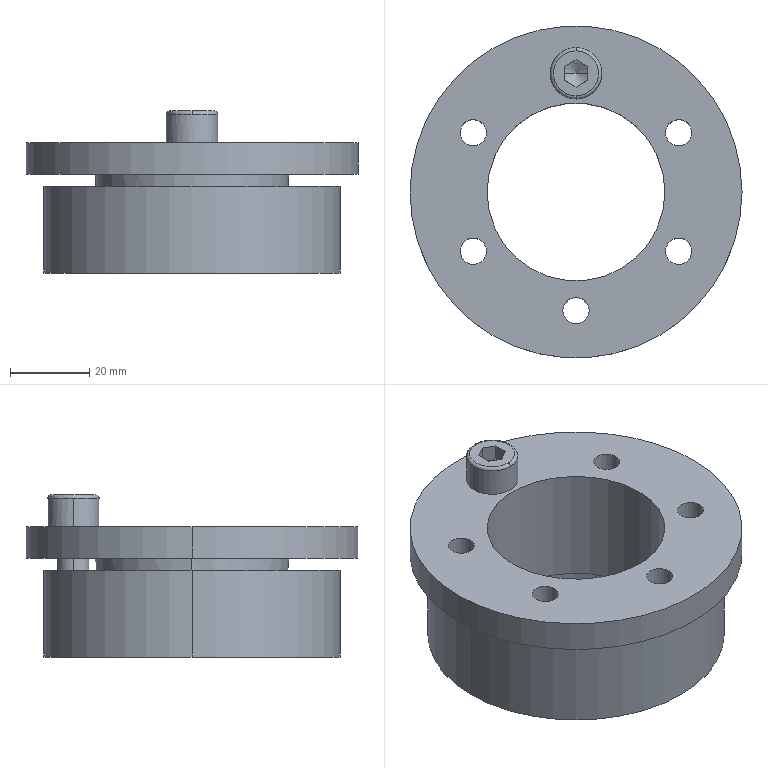Part | SolidWorks | features BaseBody 3, ICE 1 | 3 solids | 60 faces | box 84 x 84 x 41 mm | volume 89359 mm3 | cylinder 34 | plane 14 | cone 8 | torus 4 | commonest cylinder face diameters 6.647 x22 8 x2 9 x2 13 x2 45 x2 75 x2